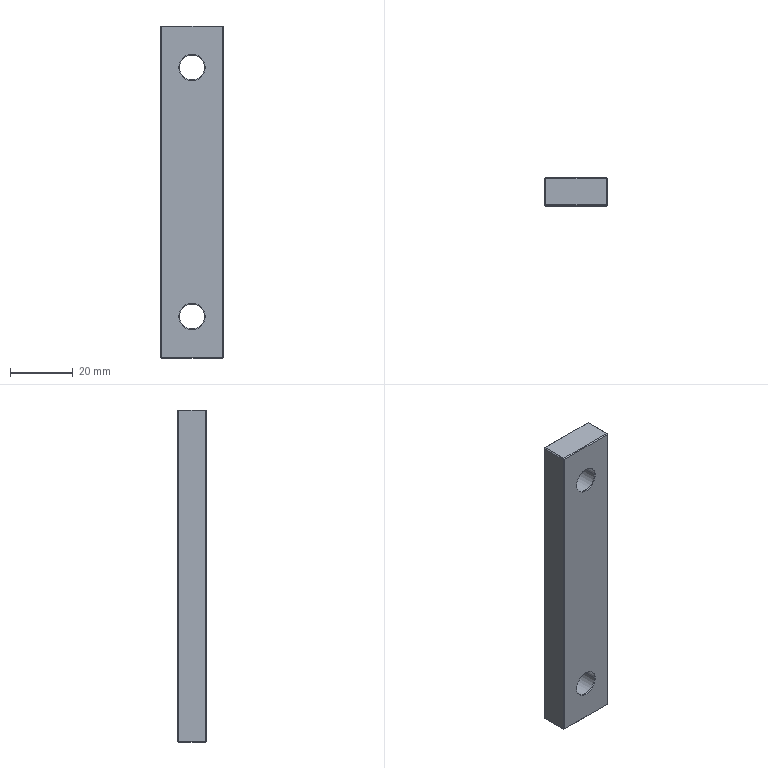Part | 1 solid | 26 faces | box 20 x 9 x 106 mm | volume 18150 mm3 | plane 18 | cylinder 4 | cone 4 | commonest cylinder face diameters 8 x4
STEP:
#1=CARTESIAN_POINT('',(2190.3,111.8,-43.5));
#2=VERTEX_POINT('',#1);
#3=CARTESIAN_POINT('',(2190.3,120.2,-43.5));
#4=VERTEX_POINT('',#3);
#5=CARTESIAN_POINT('',(2190.3,110.5,-43.5));
#6=DIRECTION('',(0.,1.,0.));
#7=VECTOR('',#6,1000.);
#8=LINE('',#5,#7);
#9=EDGE_CURVE('',#2,#4,#8,.T.);
#10=ORIENTED_EDGE('',*,*,#9,.T.);
#11=CARTESIAN_POINT('',(2209.7,120.2,-43.5));
#12=VERTEX_POINT('',#11);
#13=CARTESIAN_POINT('',(2200.,120.2,-43.5));
#14=DIRECTION('',(-1.,0.,0.));
#15=VECTOR('',#14,1000.);
#16=LINE('',#13,#15);
#17=EDGE_CURVE('',#12,#4,#16,.T.);
#18=ORIENTED_EDGE('',*,*,#17,.F.);
#19=CARTESIAN_POINT('',(2209.7,111.8,-43.5));
#20=VERTEX_POINT('',#19);
#21=CARTESIAN_POINT('',(2209.7,110.5,-43.5));
#22=DIRECTION('',(0.,-1.,0.));
#23=VECTOR('',#22,1000.);
#24=LINE('',#21,#23);
#25=EDGE_CURVE('',#12,#20,#24,.T.);
#26=ORIENTED_EDGE('',*,*,#25,.T.);
#27=CARTESIAN_POINT('',(2200.,111.8,-43.5));
#28=DIRECTION('',(1.,0.,0.));
#29=VECTOR('',#28,1000.);
#30=LINE('',#27,#29);
#31=EDGE_CURVE('',#2,#20,#30,.T.);
#32=ORIENTED_EDGE('',*,*,#31,.F.);
#33=EDGE_LOOP('',(#10,#18,#26,#32));
#34=FACE_BOUND('',#33,.T.);
#35=CARTESIAN_POINT('',(2131.5,110.5,-43.5));
#36=DIRECTION('',(0.,0.,-1.));
#37=DIRECTION('',(0.,-1.,0.));
#38=AXIS2_PLACEMENT_3D('',#35,#36,#37);
#39=PLANE('',#38);
#40=ADVANCED_FACE('',(#34),#39,.T.);
#41=CARTESIAN_POINT('',(2190.,111.8,62.2));
#42=VERTEX_POINT('',#41);
#43=CARTESIAN_POINT('',(2190.,111.8,-43.2));
#44=VERTEX_POINT('',#43);
#45=CARTESIAN_POINT('',(2190.,111.8,9.5));
#46=DIRECTION('',(0.,0.,-1.));
#47=VECTOR('',#46,1000.);
#48=LINE('',#45,#47);
#49=EDGE_CURVE('',#42,#44,#48,.T.);
#50=ORIENTED_EDGE('',*,*,#49,.F.);
#51=CARTESIAN_POINT('',(2190.,120.2,62.2));
#52=VERTEX_POINT('',#51);
#53=CARTESIAN_POINT('',(2190.,110.5,62.2));
#54=DIRECTION('',(0.,-1.,0.));
#55=VECTOR('',#54,1000.);
#56=LINE('',#53,#55);
#57=EDGE_CURVE('',#52,#42,#56,.T.);
#58=ORIENTED_EDGE('',*,*,#57,.F.);
#59=CARTESIAN_POINT('',(2190.,120.2,-43.2));
#60=VERTEX_POINT('',#59);
#61=CARTESIAN_POINT('',(2190.,120.2,9.5));
#62=DIRECTION('',(0.,0.,1.));
#63=VECTOR('',#62,1000.);
#64=LINE('',#61,#63);
#65=EDGE_CURVE('',#60,#52,#64,.T.);
#66=ORIENTED_EDGE('',*,*,#65,.F.);
#67=CARTESIAN_POINT('',(2190.,110.5,-43.2));
#68=DIRECTION('',(0.,1.,0.));
#69=VECTOR('',#68,1000.);
#70=LINE('',#67,#69);
#71=EDGE_CURVE('',#44,#60,#70,.T.);
#72=ORIENTED_EDGE('',*,*,#71,.F.);
#73=EDGE_LOOP('',(#50,#58,#66,#72));
#74=FACE_BOUND('',#73,.T.);
#75=CARTESIAN_POINT('',(2190.,110.5,62.5));
#76=DIRECTION('',(-1.,0.,0.));
#77=DIRECTION('',(0.,0.,1.));
#78=AXIS2_PLACEMENT_3D('',#75,#76,#77);
#79=PLANE('',#78);
#80=ADVANCED_FACE('',(#74),#79,.T.);
#81=CARTESIAN_POINT('',(2209.7,111.8,62.5));
#82=VERTEX_POINT('',#81);
#83=CARTESIAN_POINT('',(2209.7,120.2,62.5));
#84=VERTEX_POINT('',#83);
#85=CARTESIAN_POINT('',(2209.7,110.5,62.5));
#86=DIRECTION('',(0.,1.,0.));
#87=VECTOR('',#86,1000.);
#88=LINE('',#85,#87);
#89=EDGE_CURVE('',#82,#84,#88,.T.);
#90=ORIENTED_EDGE('',*,*,#89,.T.);
#91=CARTESIAN_POINT('',(2190.3,120.2,62.5));
#92=VERTEX_POINT('',#91);
#93=CARTESIAN_POINT('',(2200.,120.2,62.5));
#94=DIRECTION('',(-1.,0.,0.));
#95=VECTOR('',#94,1000.);
#96=LINE('',#93,#95);
#97=EDGE_CURVE('',#84,#92,#96,.T.);
#98=ORIENTED_EDGE('',*,*,#97,.T.);
#99=CARTESIAN_POINT('',(2190.3,111.8,62.5));
#100=VERTEX_POINT('',#99);
#101=CARTESIAN_POINT('',(2190.3,110.5,62.5));
#102=DIRECTION('',(0.,-1.,0.));
#103=VECTOR('',#102,1000.);
#104=LINE('',#101,#103);
#105=EDGE_CURVE('',#92,#100,#104,.T.);
#106=ORIENTED_EDGE('',*,*,#105,.T.);
#107=CARTESIAN_POINT('',(2200.,111.8,62.5));
#108=DIRECTION('',(-1.,0.,0.));
#109=VECTOR('',#108,1000.);
#110=LINE('',#107,#109);
#111=EDGE_CURVE('',#82,#100,#110,.T.);
#112=ORIENTED_EDGE('',*,*,#111,.F.);
#113=EDGE_LOOP('',(#90,#98,#106,#112));
#114=FACE_BOUND('',#113,.T.);
#115=CARTESIAN_POINT('',(2233.5,110.5,62.5));
#116=DIRECTION('',(0.,0.,1.));
#117=DIRECTION('',(1.,0.,0.));
#118=AXIS2_PLACEMENT_3D('',#115,#116,#117);
#119=PLANE('',#118);
#120=ADVANCED_FACE('',(#114),#119,.T.);
#121=CARTESIAN_POINT('',(2210.,120.2,-43.2));
#122=VERTEX_POINT('',#121);
#123=CARTESIAN_POINT('',(2210.,111.8,-43.2));
#124=VERTEX_POINT('',#123);
#125=CARTESIAN_POINT('',(2210.,110.5,-43.2));
#126=DIRECTION('',(0.,-1.,0.));
#127=VECTOR('',#126,1000.);
#128=LINE('',#125,#127);
#129=EDGE_CURVE('',#122,#124,#128,.T.);
#130=ORIENTED_EDGE('',*,*,#129,.F.);
#131=CARTESIAN_POINT('',(2210.,120.2,62.2));
#132=VERTEX_POINT('',#131);
#133=CARTESIAN_POINT('',(2210.,120.2,9.5));
#134=DIRECTION('',(0.,0.,-1.));
#135=VECTOR('',#134,1000.);
#136=LINE('',#133,#135);
#137=EDGE_CURVE('',#132,#122,#136,.T.);
#138=ORIENTED_EDGE('',*,*,#137,.F.);
#139=CARTESIAN_POINT('',(2210.,111.8,62.2));
#140=VERTEX_POINT('',#139);
#141=CARTESIAN_POINT('',(2210.,110.5,62.2));
#142=DIRECTION('',(0.,1.,0.));
#143=VECTOR('',#142,1000.);
#144=LINE('',#141,#143);
#145=EDGE_CURVE('',#140,#132,#144,.T.);
#146=ORIENTED_EDGE('',*,*,#145,.F.);
#147=CARTESIAN_POINT('',(2210.,111.8,9.5));
#148=DIRECTION('',(0.,0.,1.));
#149=VECTOR('',#148,1000.);
#150=LINE('',#147,#149);
#151=EDGE_CURVE('',#124,#140,#150,.T.);
#152=ORIENTED_EDGE('',*,*,#151,.F.);
#153=EDGE_LOOP('',(#130,#138,#146,#152));
#154=FACE_BOUND('',#153,.T.);
#155=CARTESIAN_POINT('',(2210.,110.5,-72.5));
#156=DIRECTION('',(1.,0.,0.));
#157=DIRECTION('',(0.,1.,0.));
#158=AXIS2_PLACEMENT_3D('',#155,#156,#157);
#159=PLANE('',#158);
#160=ADVANCED_FACE('',(#154),#159,.T.);
#161=CARTESIAN_POINT('',(2196.,111.7,49.25));
#162=VERTEX_POINT('',#161);
#163=CARTESIAN_POINT('',(2204.,111.7,49.25));
#164=VERTEX_POINT('',#163);
#165=CARTESIAN_POINT('',(2200.,111.7,49.25));
#166=DIRECTION('',(0.,-1.,0.));
#167=DIRECTION('',(1.,0.,0.));
#168=AXIS2_PLACEMENT_3D('',#165,#166,#167);
#169=CIRCLE('',#168,4.);
#170=EDGE_CURVE('',#162,#164,#169,.T.);
#171=ORIENTED_EDGE('',*,*,#170,.T.);
#172=CARTESIAN_POINT('',(2204.,120.5,49.25));
#173=VERTEX_POINT('',#172);
#174=CARTESIAN_POINT('',(2204.,105.5,49.25));
#175=DIRECTION('',(0.,-1.,0.));
#176=VECTOR('',#175,1000.);
#177=LINE('',#174,#176);
#178=EDGE_CURVE('',#173,#164,#177,.T.);
#179=ORIENTED_EDGE('',*,*,#178,.F.);
#180=CARTESIAN_POINT('',(2196.,120.5,49.25));
#181=VERTEX_POINT('',#180);
#182=CARTESIAN_POINT('',(2200.,120.5,49.25));
#183=DIRECTION('',(0.,-1.,0.));
#184=DIRECTION('',(1.,0.,0.));
#185=AXIS2_PLACEMENT_3D('',#182,#183,#184);
#186=CIRCLE('',#185,4.);
#187=EDGE_CURVE('',#181,#173,#186,.T.);
#188=ORIENTED_EDGE('',*,*,#187,.F.);
#189=CARTESIAN_POINT('',(2196.,105.5,49.25));
#190=DIRECTION('',(0.,-1.,0.));
#191=VECTOR('',#190,1000.);
#192=LINE('',#189,#191);
#193=EDGE_CURVE('',#181,#162,#192,.T.);
#194=ORIENTED_EDGE('',*,*,#193,.T.);
#195=EDGE_LOOP('',(#171,#179,#188,#194));
#196=FACE_BOUND('',#195,.T.);
#197=CARTESIAN_POINT('',(2200.,105.5,49.25));
#198=DIRECTION('',(0.,-1.,0.));
#199=DIRECTION('',(1.,0.,0.));
#200=AXIS2_PLACEMENT_3D('',#197,#198,#199);
#201=CYLINDRICAL_SURFACE('',#200,4.);
#202=ADVANCED_FACE('',(#196),#201,.F.);
#203=ORIENTED_EDGE('',*,*,#9,.F.);
#204=CARTESIAN_POINT('',(2190.15,111.65,-43.35));
#205=VERTEX_POINT('',#204);
#206=CARTESIAN_POINT('',(2179.688,101.188,-32.888));
#207=DIRECTION('',(0.5774,0.5774,-0.5774));
#208=VECTOR('',#207,1000.);
#209=LINE('',#206,#208);
#210=EDGE_CURVE('',#205,#2,#209,.T.);
#211=ORIENTED_EDGE('',*,*,#210,.F.);
#212=CARTESIAN_POINT('',(2191.3,110.5,-44.5));
#213=DIRECTION('',(0.5774,-0.5774,-0.5774));
#214=VECTOR('',#213,1000.);
#215=LINE('',#212,#214);
#216=EDGE_CURVE('',#44,#205,#215,.T.);
#217=ORIENTED_EDGE('',*,*,#216,.F.);
#218=ORIENTED_EDGE('',*,*,#71,.T.);
#219=CARTESIAN_POINT('',(2190.15,120.35,-43.35));
#220=VERTEX_POINT('',#219);
#221=CARTESIAN_POINT('',(2180.3,110.5,-33.5));
#222=DIRECTION('',(-0.5774,-0.5774,0.5774));
#223=VECTOR('',#222,1000.);
#224=LINE('',#221,#223);
#225=EDGE_CURVE('',#220,#60,#224,.T.);
#226=ORIENTED_EDGE('',*,*,#225,.F.);
#227=CARTESIAN_POINT('',(2200.,110.5,-53.2));
#228=DIRECTION('',(-0.5774,0.5774,0.5774));
#229=VECTOR('',#228,1000.);
#230=LINE('',#227,#229);
#231=EDGE_CURVE('',#4,#220,#230,.T.);
#232=ORIENTED_EDGE('',*,*,#231,.F.);
#233=EDGE_LOOP('',(#203,#211,#217,#218,#226,#232));
#234=FACE_BOUND('',#233,.T.);
#235=CARTESIAN_POINT('',(2190.15,114.5,-43.35));
#236=DIRECTION('',(-0.7071,0.,-0.7071));
#237=DIRECTION('',(-0.7071,0.,0.7071));
#238=AXIS2_PLACEMENT_3D('',#235,#236,#237);
#239=PLANE('',#238);
#240=ADVANCED_FACE('',(#234),#239,.T.);
#241=ORIENTED_EDGE('',*,*,#57,.T.);
#242=CARTESIAN_POINT('',(2190.15,111.65,62.35));
#243=VERTEX_POINT('',#242);
#244=CARTESIAN_POINT('',(2191.3,110.5,63.5));
#245=DIRECTION('',(0.5774,-0.5774,0.5774));
#246=VECTOR('',#245,1000.);
#247=LINE('',#244,#246);
#248=EDGE_CURVE('',#42,#243,#247,.T.);
#249=ORIENTED_EDGE('',*,*,#248,.T.);
#250=CARTESIAN_POINT('',(2189.,110.5,61.2));
#251=DIRECTION('',(0.5774,0.5774,0.5774));
#252=VECTOR('',#251,1000.);
#253=LINE('',#250,#252);
#254=EDGE_CURVE('',#243,#100,#253,.T.);
#255=ORIENTED_EDGE('',*,*,#254,.T.);
#256=ORIENTED_EDGE('',*,*,#105,.F.);
#257=CARTESIAN_POINT('',(2190.15,120.35,62.35));
#258=VERTEX_POINT('',#257);
#259=CARTESIAN_POINT('',(2200.,110.5,72.2));
#260=DIRECTION('',(-0.5774,0.5774,-0.5774));
#261=VECTOR('',#260,1000.);
#262=LINE('',#259,#261);
#263=EDGE_CURVE('',#92,#258,#262,.T.);
#264=ORIENTED_EDGE('',*,*,#263,.T.);
#265=CARTESIAN_POINT('',(2180.3,110.5,52.5));
#266=DIRECTION('',(0.5774,0.5774,0.5774));
#267=VECTOR('',#266,1000.);
#268=LINE('',#265,#267);
#269=EDGE_CURVE('',#52,#258,#268,.T.);
#270=ORIENTED_EDGE('',*,*,#269,.F.);
#271=EDGE_LOOP('',(#241,#249,#255,#256,#264,#270));
#272=FACE_BOUND('',#271,.T.);
#273=CARTESIAN_POINT('',(2190.15,114.5,62.35));
#274=DIRECTION('',(0.7071,0.,-0.7071));
#275=DIRECTION('',(0.,-1.,0.));
#276=AXIS2_PLACEMENT_3D('',#273,#274,#275);
#277=PLANE('',#276);
#278=ADVANCED_FACE('',(#272),#277,.F.);
#279=ORIENTED_EDGE('',*,*,#89,.F.);
#280=CARTESIAN_POINT('',(2209.85,111.65,62.35));
#281=VERTEX_POINT('',#280);
#282=CARTESIAN_POINT('',(2211.,110.5,61.2));
#283=DIRECTION('',(-0.5774,0.5774,0.5774));
#284=VECTOR('',#283,1000.);
#285=LINE('',#282,#284);
#286=EDGE_CURVE('',#281,#82,#285,.T.);
#287=ORIENTED_EDGE('',*,*,#286,.F.);
#288=CARTESIAN_POINT('',(2305.088,206.888,-32.888));
#289=DIRECTION('',(-0.5774,-0.5774,0.5774));
#290=VECTOR('',#289,1000.);
#291=LINE('',#288,#290);
#292=EDGE_CURVE('',#140,#281,#291,.T.);
#293=ORIENTED_EDGE('',*,*,#292,.F.);
#294=ORIENTED_EDGE('',*,*,#145,.T.);
#295=CARTESIAN_POINT('',(2209.85,120.35,62.35));
#296=VERTEX_POINT('',#295);
#297=CARTESIAN_POINT('',(2305.088,25.112,-32.888));
#298=DIRECTION('',(-0.5774,0.5774,0.5774));
#299=VECTOR('',#298,1000.);
#300=LINE('',#297,#299);
#301=EDGE_CURVE('',#132,#296,#300,.T.);
#302=ORIENTED_EDGE('',*,*,#301,.T.);
#303=CARTESIAN_POINT('',(2200.,110.5,72.2));
#304=DIRECTION('',(-0.5774,-0.5774,0.5774));
#305=VECTOR('',#304,1000.);
#306=LINE('',#303,#305);
#307=EDGE_CURVE('',#296,#84,#306,.T.);
#308=ORIENTED_EDGE('',*,*,#307,.T.);
#309=EDGE_LOOP('',(#279,#287,#293,#294,#302,#308));
#310=FACE_BOUND('',#309,.T.);
#311=CARTESIAN_POINT('',(2209.85,114.5,62.35));
#312=DIRECTION('',(0.7071,0.,0.7071));
#313=DIRECTION('',(0.,-1.,0.));
#314=AXIS2_PLACEMENT_3D('',#311,#312,#313);
#315=PLANE('',#314);
#316=ADVANCED_FACE('',(#310),#315,.T.);
#317=ORIENTED_EDGE('',*,*,#129,.T.);
#318=CARTESIAN_POINT('',(2209.85,111.65,-43.35));
#319=VERTEX_POINT('',#318);
#320=CARTESIAN_POINT('',(2220.312,122.112,-32.888));
#321=DIRECTION('',(0.5774,0.5774,0.5774));
#322=VECTOR('',#321,1000.);
#323=LINE('',#320,#322);
#324=EDGE_CURVE('',#319,#124,#323,.T.);
#325=ORIENTED_EDGE('',*,*,#324,.F.);
#326=CARTESIAN_POINT('',(2220.312,101.188,-32.888));
#327=DIRECTION('',(0.5774,-0.5774,0.5774));
#328=VECTOR('',#327,1000.);
#329=LINE('',#326,#328);
#330=EDGE_CURVE('',#20,#319,#329,.T.);
#331=ORIENTED_EDGE('',*,*,#330,.F.);
#332=ORIENTED_EDGE('',*,*,#25,.F.);
#333=CARTESIAN_POINT('',(2209.85,120.35,-43.35));
#334=VERTEX_POINT('',#333);
#335=CARTESIAN_POINT('',(2220.312,130.812,-32.888));
#336=DIRECTION('',(0.5774,0.5774,0.5774));
#337=VECTOR('',#336,1000.);
#338=LINE('',#335,#337);
#339=EDGE_CURVE('',#12,#334,#338,.T.);
#340=ORIENTED_EDGE('',*,*,#339,.T.);
#341=CARTESIAN_POINT('',(2220.312,109.888,-32.888));
#342=DIRECTION('',(-0.5774,0.5774,-0.5774));
#343=VECTOR('',#342,1000.);
#344=LINE('',#341,#343);
#345=EDGE_CURVE('',#122,#334,#344,.T.);
#346=ORIENTED_EDGE('',*,*,#345,.F.);
#347=EDGE_LOOP('',(#317,#325,#331,#332,#340,#346));
#348=FACE_BOUND('',#347,.T.);
#349=CARTESIAN_POINT('',(2209.85,114.5,-43.35));
#350=DIRECTION('',(0.7071,0.,-0.7071));
#351=DIRECTION('',(0.,-1.,0.));
#352=AXIS2_PLACEMENT_3D('',#349,#350,#351);
#353=PLANE('',#352);
#354=ADVANCED_FACE('',(#348),#353,.T.);
#355=ORIENTED_EDGE('',*,*,#170,.F.);
#356=CARTESIAN_POINT('',(2195.8,111.5,49.25));
#357=VERTEX_POINT('',#356);
#358=CARTESIAN_POINT('',(2196.,111.7,49.25));
#359=DIRECTION('',(-0.7071,-0.7071,0.));
#360=VECTOR('',#359,1000.);
#361=LINE('',#358,#360);
#362=EDGE_CURVE('',#162,#357,#361,.T.);
#363=ORIENTED_EDGE('',*,*,#362,.T.);
#364=CARTESIAN_POINT('',(2204.2,111.5,49.25));
#365=VERTEX_POINT('',#364);
#366=CARTESIAN_POINT('',(2200.,111.5,49.25));
#367=DIRECTION('',(0.,-1.,0.));
#368=DIRECTION('',(1.,0.,0.));
#369=AXIS2_PLACEMENT_3D('',#366,#367,#368);
#370=CIRCLE('',#369,4.2);
#371=EDGE_CURVE('',#357,#365,#370,.T.);
#372=ORIENTED_EDGE('',*,*,#371,.T.);
#373=CARTESIAN_POINT('',(2204.,111.7,49.25));
#374=DIRECTION('',(0.7071,-0.7071,0.));
#375=VECTOR('',#374,1000.);
#376=LINE('',#373,#375);
#377=EDGE_CURVE('',#164,#365,#376,.T.);
#378=ORIENTED_EDGE('',*,*,#377,.F.);
#379=EDGE_LOOP('',(#355,#363,#372,#378));
#380=FACE_BOUND('',#379,.T.);
#381=CARTESIAN_POINT('',(2200.,111.7,49.25));
#382=DIRECTION('',(0.,-1.,0.));
#383=DIRECTION('',(1.,0.,0.));
#384=AXIS2_PLACEMENT_3D('',#381,#382,#383);
#385=CONICAL_SURFACE('',#384,4.,0.7854);
#386=ADVANCED_FACE('',(#380),#385,.F.);
#387=ORIENTED_EDGE('',*,*,#178,.T.);
#388=CARTESIAN_POINT('',(2200.,111.7,49.25));
#389=DIRECTION('',(0.,-1.,0.));
#390=DIRECTION('',(1.,0.,0.));
#391=AXIS2_PLACEMENT_3D('',#388,#389,#390);
#392=CIRCLE('',#391,4.);
#393=EDGE_CURVE('',#164,#162,#392,.T.);
#394=ORIENTED_EDGE('',*,*,#393,.T.);
#395=ORIENTED_EDGE('',*,*,#193,.F.);
#396=CARTESIAN_POINT('',(2200.,120.5,49.25));
#397=DIRECTION('',(0.,-1.,0.));
#398=DIRECTION('',(1.,0.,0.));
#399=AXIS2_PLACEMENT_3D('',#396,#397,#398);
#400=CIRCLE('',#399,4.);
#401=EDGE_CURVE('',#173,#181,#400,.T.);
#402=ORIENTED_EDGE('',*,*,#401,.F.);
#403=EDGE_LOOP('',(#387,#394,#395,#402));
#404=FACE_BOUND('',#403,.T.);
#405=CARTESIAN_POINT('',(2200.,105.5,49.25));
#406=DIRECTION('',(0.,-1.,0.));
#407=DIRECTION('',(1.,0.,0.));
#408=AXIS2_PLACEMENT_3D('',#405,#406,#407);
#409=CYLINDRICAL_SURFACE('',#408,4.);
#410=ADVANCED_FACE('',(#404),#409,.F.);
#411=ORIENTED_EDGE('',*,*,#377,.T.);
#412=CARTESIAN_POINT('',(2200.,111.5,49.25));
#413=DIRECTION('',(0.,-1.,0.));
#414=DIRECTION('',(1.,0.,0.));
#415=AXIS2_PLACEMENT_3D('',#412,#413,#414);
#416=CIRCLE('',#415,4.2);
#417=EDGE_CURVE('',#365,#357,#416,.T.);
#418=ORIENTED_EDGE('',*,*,#417,.T.);
#419=ORIENTED_EDGE('',*,*,#362,.F.);
#420=ORIENTED_EDGE('',*,*,#393,.F.);
#421=EDGE_LOOP('',(#411,#418,#419,#420));
#422=FACE_BOUND('',#421,.T.);
#423=CARTESIAN_POINT('',(2200.,111.7,49.25));
#424=DIRECTION('',(0.,-1.,0.));
#425=DIRECTION('',(1.,0.,0.));
#426=AXIS2_PLACEMENT_3D('',#423,#424,#425);
#427=CONICAL_SURFACE('',#426,4.,0.7854);
#428=ADVANCED_FACE('',(#422),#427,.F.);
#429=CARTESIAN_POINT('',(2209.7,120.5,-43.2));
#430=VERTEX_POINT('',#429);
#431=CARTESIAN_POINT('',(2190.3,120.5,-43.2));
#432=VERTEX_POINT('',#431);
#433=CARTESIAN_POINT('',(2200.,120.5,-43.2));
#434=DIRECTION('',(-1.,0.,0.));
#435=VECTOR('',#434,1000.);
#436=LINE('',#433,#435);
#437=EDGE_CURVE('',#430,#432,#436,.T.);
#438=ORIENTED_EDGE('',*,*,#437,.T.);
#439=CARTESIAN_POINT('',(2190.3,120.5,62.2));
#440=VERTEX_POINT('',#439);
#441=CARTESIAN_POINT('',(2190.3,120.5,9.5));
#442=DIRECTION('',(0.,0.,1.));
#443=VECTOR('',#442,1000.);
#444=LINE('',#441,#443);
#445=EDGE_CURVE('',#432,#440,#444,.T.);
#446=ORIENTED_EDGE('',*,*,#445,.T.);
#447=CARTESIAN_POINT('',(2209.7,120.5,62.2));
#448=VERTEX_POINT('',#447);
#449=CARTESIAN_POINT('',(2200.,120.5,62.2));
#450=DIRECTION('',(-1.,0.,0.));
#451=VECTOR('',#450,1000.);
#452=LINE('',#449,#451);
#453=EDGE_CURVE('',#448,#440,#452,.T.);
#454=ORIENTED_EDGE('',*,*,#453,.F.);
#455=CARTESIAN_POINT('',(2209.7,120.5,9.5));
#456=DIRECTION('',(0.,0.,-1.));
#457=VECTOR('',#456,1000.);
#458=LINE('',#455,#457);
#459=EDGE_CURVE('',#448,#430,#458,.T.);
#460=ORIENTED_EDGE('',*,*,#459,.T.);
#461=EDGE_LOOP('',(#438,#446,#454,#460));
#462=FACE_BOUND('',#461,.T.);
#463=ORIENTED_EDGE('',*,*,#187,.T.);
#464=ORIENTED_EDGE('',*,*,#401,.T.);
#465=EDGE_LOOP('',(#463,#464));
#466=FACE_BOUND('',#465,.T.);
#467=CARTESIAN_POINT('',(2196.,120.5,-30.25));
#468=VERTEX_POINT('',#467);
#469=CARTESIAN_POINT('',(2204.,120.5,-30.25));
#470=VERTEX_POINT('',#469);
#471=CARTESIAN_POINT('',(2200.,120.5,-30.25));
#472=DIRECTION('',(0.,-1.,0.));
#473=DIRECTION('',(1.,0.,0.));
#474=AXIS2_PLACEMENT_3D('',#471,#472,#473);
#475=CIRCLE('',#474,4.);
#476=EDGE_CURVE('',#468,#470,#475,.T.);
#477=ORIENTED_EDGE('',*,*,#476,.T.);
#478=CARTESIAN_POINT('',(2200.,120.5,-30.25));
#479=DIRECTION('',(0.,-1.,0.));
#480=DIRECTION('',(1.,0.,0.));
#481=AXIS2_PLACEMENT_3D('',#478,#479,#480);
#482=CIRCLE('',#481,4.);
#483=EDGE_CURVE('',#470,#468,#482,.T.);
#484=ORIENTED_EDGE('',*,*,#483,.T.);
#485=EDGE_LOOP('',(#477,#484));
#486=FACE_BOUND('',#485,.T.);
#487=CARTESIAN_POINT('',(2184.262,120.5,-32.888));
#488=DIRECTION('',(0.,1.,0.));
#489=DIRECTION('',(1.,0.,0.));
#490=AXIS2_PLACEMENT_3D('',#487,#488,#489);
#491=PLANE('',#490);
#492=ADVANCED_FACE('',(#462,#466,#486),#491,.T.);
#493=CARTESIAN_POINT('',(2196.,111.7,-30.25));
#494=VERTEX_POINT('',#493);
#495=CARTESIAN_POINT('',(2204.,111.7,-30.25));
#496=VERTEX_POINT('',#495);
#497=CARTESIAN_POINT('',(2200.,111.7,-30.25));
#498=DIRECTION('',(0.,-1.,0.));
#499=DIRECTION('',(1.,0.,0.));
#500=AXIS2_PLACEMENT_3D('',#497,#498,#499);
#501=CIRCLE('',#500,4.);
#502=EDGE_CURVE('',#494,#496,#501,.T.);
#503=ORIENTED_EDGE('',*,*,#502,.T.);
#504=CARTESIAN_POINT('',(2204.,105.5,-30.25));
#505=DIRECTION('',(0.,-1.,0.));
#506=VECTOR('',#505,1000.);
#507=LINE('',#504,#506);
#508=EDGE_CURVE('',#470,#496,#507,.T.);
#509=ORIENTED_EDGE('',*,*,#508,.F.);
#510=ORIENTED_EDGE('',*,*,#476,.F.);
#511=CARTESIAN_POINT('',(2196.,105.5,-30.25));
#512=DIRECTION('',(0.,-1.,0.));
#513=VECTOR('',#512,1000.);
#514=LINE('',#511,#513);
#515=EDGE_CURVE('',#468,#494,#514,.T.);
#516=ORIENTED_EDGE('',*,*,#515,.T.);
#517=EDGE_LOOP('',(#503,#509,#510,#516));
#518=FACE_BOUND('',#517,.T.);
#519=CARTESIAN_POINT('',(2200.,105.5,-30.25));
#520=DIRECTION('',(0.,-1.,0.));
#521=DIRECTION('',(1.,0.,0.));
#522=AXIS2_PLACEMENT_3D('',#519,#520,#521);
#523=CYLINDRICAL_SURFACE('',#522,4.);
#524=ADVANCED_FACE('',(#518),#523,.F.);
#525=ORIENTED_EDGE('',*,*,#437,.F.);
#526=CARTESIAN_POINT('',(2219.7,110.5,-53.2));
#527=DIRECTION('',(-0.5774,0.5774,0.5774));
#528=VECTOR('',#527,1000.);
#529=LINE('',#526,#528);
#530=EDGE_CURVE('',#334,#430,#529,.T.);
#531=ORIENTED_EDGE('',*,*,#530,.F.);
#532=ORIENTED_EDGE('',*,*,#339,.F.);
#533=ORIENTED_EDGE('',*,*,#17,.T.);
#534=ORIENTED_EDGE('',*,*,#231,.T.);
#535=CARTESIAN_POINT('',(2180.3,110.5,-53.2));
#536=DIRECTION('',(-0.5774,-0.5774,-0.5774));
#537=VECTOR('',#536,1000.);
#538=LINE('',#535,#537);
#539=EDGE_CURVE('',#432,#220,#538,.T.);
#540=ORIENTED_EDGE('',*,*,#539,.F.);
#541=EDGE_LOOP('',(#525,#531,#532,#533,#534,#540));
#542=FACE_BOUND('',#541,.T.);
#543=CARTESIAN_POINT('',(2200.,120.35,-43.35));
#544=DIRECTION('',(0.,0.7071,-0.7071));
#545=DIRECTION('',(-1.,0.,0.));
#546=AXIS2_PLACEMENT_3D('',#543,#544,#545);
#547=PLANE('',#546);
#548=ADVANCED_FACE('',(#542),#547,.T.);
#549=ORIENTED_EDGE('',*,*,#453,.T.);
#550=CARTESIAN_POINT('',(2180.3,110.5,72.2));
#551=DIRECTION('',(0.5774,0.5774,-0.5774));
#552=VECTOR('',#551,1000.);
#553=LINE('',#550,#552);
#554=EDGE_CURVE('',#258,#440,#553,.T.);
#555=ORIENTED_EDGE('',*,*,#554,.F.);
#556=ORIENTED_EDGE('',*,*,#263,.F.);
#557=ORIENTED_EDGE('',*,*,#97,.F.);
#558=ORIENTED_EDGE('',*,*,#307,.F.);
#559=CARTESIAN_POINT('',(2219.7,110.5,72.2));
#560=DIRECTION('',(0.5774,-0.5774,0.5774));
#561=VECTOR('',#560,1000.);
#562=LINE('',#559,#561);
#563=EDGE_CURVE('',#448,#296,#562,.T.);
#564=ORIENTED_EDGE('',*,*,#563,.F.);
#565=EDGE_LOOP('',(#549,#555,#556,#557,#558,#564));
#566=FACE_BOUND('',#565,.T.);
#567=CARTESIAN_POINT('',(2200.,120.35,62.35));
#568=DIRECTION('',(0.,-0.7071,-0.7071));
#569=DIRECTION('',(0.,-0.7071,0.7071));
#570=AXIS2_PLACEMENT_3D('',#567,#568,#569);
#571=PLANE('',#570);
#572=ADVANCED_FACE('',(#566),#571,.F.);
#573=ORIENTED_EDGE('',*,*,#445,.F.);
#574=ORIENTED_EDGE('',*,*,#539,.T.);
#575=ORIENTED_EDGE('',*,*,#225,.T.);
#576=ORIENTED_EDGE('',*,*,#65,.T.);
#577=ORIENTED_EDGE('',*,*,#269,.T.);
#578=ORIENTED_EDGE('',*,*,#554,.T.);
#579=EDGE_LOOP('',(#573,#574,#575,#576,#577,#578));
#580=FACE_BOUND('',#579,.T.);
#581=CARTESIAN_POINT('',(2190.15,120.35,9.5));
#582=DIRECTION('',(-0.7071,0.7071,0.));
#583=DIRECTION('',(0.,0.,1.));
#584=AXIS2_PLACEMENT_3D('',#581,#582,#583);
#585=PLANE('',#584);
#586=ADVANCED_FACE('',(#580),#585,.T.);
#587=ORIENTED_EDGE('',*,*,#459,.F.);
#588=ORIENTED_EDGE('',*,*,#563,.T.);
#589=ORIENTED_EDGE('',*,*,#301,.F.);
#590=ORIENTED_EDGE('',*,*,#137,.T.);
#591=ORIENTED_EDGE('',*,*,#345,.T.);
#592=ORIENTED_EDGE('',*,*,#530,.T.);
#593=EDGE_LOOP('',(#587,#588,#589,#590,#591,#592));
#594=FACE_BOUND('',#593,.T.);
#595=CARTESIAN_POINT('',(2209.85,120.35,9.5));
#596=DIRECTION('',(0.7071,0.7071,0.));
#597=DIRECTION('',(0.,0.,-1.));
#598=AXIS2_PLACEMENT_3D('',#595,#596,#597);
#599=PLANE('',#598);
#600=ADVANCED_FACE('',(#594),#599,.T.);
#601=ORIENTED_EDGE('',*,*,#502,.F.);
#602=CARTESIAN_POINT('',(2195.8,111.5,-30.25));
#603=VERTEX_POINT('',#602);
#604=CARTESIAN_POINT('',(2196.,111.7,-30.25));
#605=DIRECTION('',(-0.7071,-0.7071,0.));
#606=VECTOR('',#605,1000.);
#607=LINE('',#604,#606);
#608=EDGE_CURVE('',#494,#603,#607,.T.);
#609=ORIENTED_EDGE('',*,*,#608,.T.);
#610=CARTESIAN_POINT('',(2204.2,111.5,-30.25));
#611=VERTEX_POINT('',#610);
#612=CARTESIAN_POINT('',(2200.,111.5,-30.25));
#613=DIRECTION('',(0.,-1.,0.));
#614=DIRECTION('',(1.,0.,0.));
#615=AXIS2_PLACEMENT_3D('',#612,#613,#614);
#616=CIRCLE('',#615,4.2);
#617=EDGE_CURVE('',#603,#611,#616,.T.);
#618=ORIENTED_EDGE('',*,*,#617,.T.);
#619=CARTESIAN_POINT('',(2204.,111.7,-30.25));
#620=DIRECTION('',(0.7071,-0.7071,0.));
#621=VECTOR('',#620,1000.);
#622=LINE('',#619,#621);
#623=EDGE_CURVE('',#496,#611,#622,.T.);
#624=ORIENTED_EDGE('',*,*,#623,.F.);
#625=EDGE_LOOP('',(#601,#609,#618,#624));
#626=FACE_BOUND('',#625,.T.);
#627=CARTESIAN_POINT('',(2200.,111.7,-30.25));
#628=DIRECTION('',(0.,-1.,0.));
#629=DIRECTION('',(1.,0.,0.));
#630=AXIS2_PLACEMENT_3D('',#627,#628,#629);
#631=CONICAL_SURFACE('',#630,4.,0.7854);
#632=ADVANCED_FACE('',(#626),#631,.F.);
#633=ORIENTED_EDGE('',*,*,#508,.T.);
#634=CARTESIAN_POINT('',(2200.,111.7,-30.25));
#635=DIRECTION('',(0.,-1.,0.));
#636=DIRECTION('',(1.,0.,0.));
#637=AXIS2_PLACEMENT_3D('',#634,#635,#636);
#638=CIRCLE('',#637,4.);
#639=EDGE_CURVE('',#496,#494,#638,.T.);
#640=ORIENTED_EDGE('',*,*,#639,.T.);
#641=ORIENTED_EDGE('',*,*,#515,.F.);
#642=ORIENTED_EDGE('',*,*,#483,.F.);
#643=EDGE_LOOP('',(#633,#640,#641,#642));
#644=FACE_BOUND('',#643,.T.);
#645=CARTESIAN_POINT('',(2200.,105.5,-30.25));
#646=DIRECTION('',(0.,-1.,0.));
#647=DIRECTION('',(1.,0.,0.));
#648=AXIS2_PLACEMENT_3D('',#645,#646,#647);
#649=CYLINDRICAL_SURFACE('',#648,4.);
#650=ADVANCED_FACE('',(#644),#649,.F.);
#651=ORIENTED_EDGE('',*,*,#623,.T.);
#652=CARTESIAN_POINT('',(2200.,111.5,-30.25));
#653=DIRECTION('',(0.,-1.,0.));
#654=DIRECTION('',(1.,0.,0.));
#655=AXIS2_PLACEMENT_3D('',#652,#653,#654);
#656=CIRCLE('',#655,4.2);
#657=EDGE_CURVE('',#611,#603,#656,.T.);
#658=ORIENTED_EDGE('',*,*,#657,.T.);
#659=ORIENTED_EDGE('',*,*,#608,.F.);
#660=ORIENTED_EDGE('',*,*,#639,.F.);
#661=EDGE_LOOP('',(#651,#658,#659,#660));
#662=FACE_BOUND('',#661,.T.);
#663=CARTESIAN_POINT('',(2200.,111.7,-30.25));
#664=DIRECTION('',(0.,-1.,0.));
#665=DIRECTION('',(1.,0.,0.));
#666=AXIS2_PLACEMENT_3D('',#663,#664,#665);
#667=CONICAL_SURFACE('',#666,4.,0.7854);
#668=ADVANCED_FACE('',(#662),#667,.F.);
#669=CARTESIAN_POINT('',(2190.3,111.5,-43.2));
#670=VERTEX_POINT('',#669);
#671=CARTESIAN_POINT('',(2209.7,111.5,-43.2));
#672=VERTEX_POINT('',#671);
#673=CARTESIAN_POINT('',(2200.,111.5,-43.2));
#674=DIRECTION('',(1.,0.,0.));
#675=VECTOR('',#674,1000.);
#676=LINE('',#673,#675);
#677=EDGE_CURVE('',#670,#672,#676,.T.);
#678=ORIENTED_EDGE('',*,*,#677,.T.);
#679=CARTESIAN_POINT('',(2209.7,111.5,62.2));
#680=VERTEX_POINT('',#679);
#681=CARTESIAN_POINT('',(2209.7,111.5,9.5));
#682=DIRECTION('',(0.,0.,1.));
#683=VECTOR('',#682,1000.);
#684=LINE('',#681,#683);
#685=EDGE_CURVE('',#672,#680,#684,.T.);
#686=ORIENTED_EDGE('',*,*,#685,.T.);
#687=CARTESIAN_POINT('',(2190.3,111.5,62.2));
#688=VERTEX_POINT('',#687);
#689=CARTESIAN_POINT('',(2200.,111.5,62.2));
#690=DIRECTION('',(-1.,0.,0.));
#691=VECTOR('',#690,1000.);
#692=LINE('',#689,#691);
#693=EDGE_CURVE('',#680,#688,#692,.T.);
#694=ORIENTED_EDGE('',*,*,#693,.T.);
#695=CARTESIAN_POINT('',(2190.3,111.5,9.5));
#696=DIRECTION('',(0.,0.,-1.));
#697=VECTOR('',#696,1000.);
#698=LINE('',#695,#697);
#699=EDGE_CURVE('',#688,#670,#698,.T.);
#700=ORIENTED_EDGE('',*,*,#699,.T.);
#701=EDGE_LOOP('',(#678,#686,#694,#700));
#702=FACE_BOUND('',#701,.T.);
#703=ORIENTED_EDGE('',*,*,#371,.F.);
#704=ORIENTED_EDGE('',*,*,#417,.F.);
#705=EDGE_LOOP('',(#703,#704));
#706=FACE_BOUND('',#705,.T.);
#707=ORIENTED_EDGE('',*,*,#617,.F.);
#708=ORIENTED_EDGE('',*,*,#657,.F.);
#709=EDGE_LOOP('',(#707,#708));
#710=FACE_BOUND('',#709,.T.);
#711=CARTESIAN_POINT('',(2184.262,111.5,-32.888));
#712=DIRECTION('',(0.,1.,0.));
#713=DIRECTION('',(1.,0.,0.));
#714=AXIS2_PLACEMENT_3D('',#711,#712,#713);
#715=PLANE('',#714);
#716=ADVANCED_FACE('',(#702,#706,#710),#715,.F.);
#717=ORIENTED_EDGE('',*,*,#699,.F.);
#718=CARTESIAN_POINT('',(2191.3,110.5,61.2));
#719=DIRECTION('',(0.5774,-0.5774,-0.5774));
#720=VECTOR('',#719,1000.);
#721=LINE('',#718,#720);
#722=EDGE_CURVE('',#243,#688,#721,.T.);
#723=ORIENTED_EDGE('',*,*,#722,.F.);
#724=ORIENTED_EDGE('',*,*,#248,.F.);
#725=ORIENTED_EDGE('',*,*,#49,.T.);
#726=ORIENTED_EDGE('',*,*,#216,.T.);
#727=CARTESIAN_POINT('',(2200.612,101.188,-32.888));
#728=DIRECTION('',(-0.5774,0.5774,-0.5774));
#729=VECTOR('',#728,1000.);
#730=LINE('',#727,#729);
#731=EDGE_CURVE('',#670,#205,#730,.T.);
#732=ORIENTED_EDGE('',*,*,#731,.F.);
#733=EDGE_LOOP('',(#717,#723,#724,#725,#726,#732));
#734=FACE_BOUND('',#733,.T.);
#735=CARTESIAN_POINT('',(2190.15,111.65,9.5));
#736=DIRECTION('',(-0.7071,-0.7071,0.));
#737=DIRECTION('',(-0.7071,0.7071,0.));
#738=AXIS2_PLACEMENT_3D('',#735,#736,#737);
#739=PLANE('',#738);
#740=ADVANCED_FACE('',(#734),#739,.T.);
#741=ORIENTED_EDGE('',*,*,#693,.F.);
#742=CARTESIAN_POINT('',(2184.262,86.062,36.762));
#743=DIRECTION('',(-0.5774,-0.5774,-0.5774));
#744=VECTOR('',#743,1000.);
#745=LINE('',#742,#744);
#746=EDGE_CURVE('',#281,#680,#745,.T.);
#747=ORIENTED_EDGE('',*,*,#746,.F.);
#748=ORIENTED_EDGE('',*,*,#286,.T.);
#749=ORIENTED_EDGE('',*,*,#111,.T.);
#750=ORIENTED_EDGE('',*,*,#254,.F.);
#751=ORIENTED_EDGE('',*,*,#722,.T.);
#752=EDGE_LOOP('',(#741,#747,#748,#749,#750,#751));
#753=FACE_BOUND('',#752,.T.);
#754=CARTESIAN_POINT('',(2200.,111.65,62.35));
#755=DIRECTION('',(0.,-0.7071,0.7071));
#756=DIRECTION('',(-1.,0.,0.));
#757=AXIS2_PLACEMENT_3D('',#754,#755,#756);
#758=PLANE('',#757);
#759=ADVANCED_FACE('',(#753),#758,.T.);
#760=ORIENTED_EDGE('',*,*,#685,.F.);
#761=CARTESIAN_POINT('',(2199.388,101.188,-32.888));
#762=DIRECTION('',(-0.5774,-0.5774,0.5774));
#763=VECTOR('',#762,1000.);
#764=LINE('',#761,#763);
#765=EDGE_CURVE('',#319,#672,#764,.T.);
#766=ORIENTED_EDGE('',*,*,#765,.F.);
#767=ORIENTED_EDGE('',*,*,#324,.T.);
#768=ORIENTED_EDGE('',*,*,#151,.T.);
#769=ORIENTED_EDGE('',*,*,#292,.T.);
#770=ORIENTED_EDGE('',*,*,#746,.T.);
#771=EDGE_LOOP('',(#760,#766,#767,#768,#769,#770));
#772=FACE_BOUND('',#771,.T.);
#773=CARTESIAN_POINT('',(2209.85,111.65,9.5));
#774=DIRECTION('',(0.7071,-0.7071,0.));
#775=DIRECTION('',(0.,0.,-1.));
#776=AXIS2_PLACEMENT_3D('',#773,#774,#775);
#777=PLANE('',#776);
#778=ADVANCED_FACE('',(#772),#777,.T.);
#779=ORIENTED_EDGE('',*,*,#677,.F.);
#780=ORIENTED_EDGE('',*,*,#731,.T.);
#781=ORIENTED_EDGE('',*,*,#210,.T.);
#782=ORIENTED_EDGE('',*,*,#31,.T.);
#783=ORIENTED_EDGE('',*,*,#330,.T.);
#784=ORIENTED_EDGE('',*,*,#765,.T.);
#785=EDGE_LOOP('',(#779,#780,#781,#782,#783,#784));
#786=FACE_BOUND('',#785,.T.);
#787=CARTESIAN_POINT('',(2200.,111.65,-43.35));
#788=DIRECTION('',(0.,-0.7071,-0.7071));
#789=DIRECTION('',(0.,0.7071,-0.7071));
#790=AXIS2_PLACEMENT_3D('',#787,#788,#789);
#791=PLANE('',#790);
#792=ADVANCED_FACE('',(#786),#791,.T.);
#793=CLOSED_SHELL('',(#40,#80,#120,#160,#202,#240,#278,#316,#354,#386,#410,#428,#492,#524,#548,#572,#586,#600,#632,#650,#668,#716,#740,#759,#778,#792));
#794=MANIFOLD_SOLID_BREP('',#793);
#795=(LENGTH_UNIT()NAMED_UNIT(*)SI_UNIT(.MILLI.,.METRE.));
#796=UNCERTAINTY_MEASURE_WITH_UNIT(LENGTH_MEASURE(0.00001),#795,'','');
#797=(NAMED_UNIT(*)PLANE_ANGLE_UNIT()SI_UNIT($,.RADIAN.));
#798=(NAMED_UNIT(*)SI_UNIT($,.STERADIAN.)SOLID_ANGLE_UNIT());
#799=(GEOMETRIC_REPRESENTATION_CONTEXT(3)GLOBAL_UNCERTAINTY_ASSIGNED_CONTEXT((#796))GLOBAL_UNIT_ASSIGNED_CONTEXT((#795,#797,#798))REPRESENTATION_CONTEXT('',''));
#800=ADVANCED_BREP_SHAPE_REPRESENTATION('',(#794),#799);